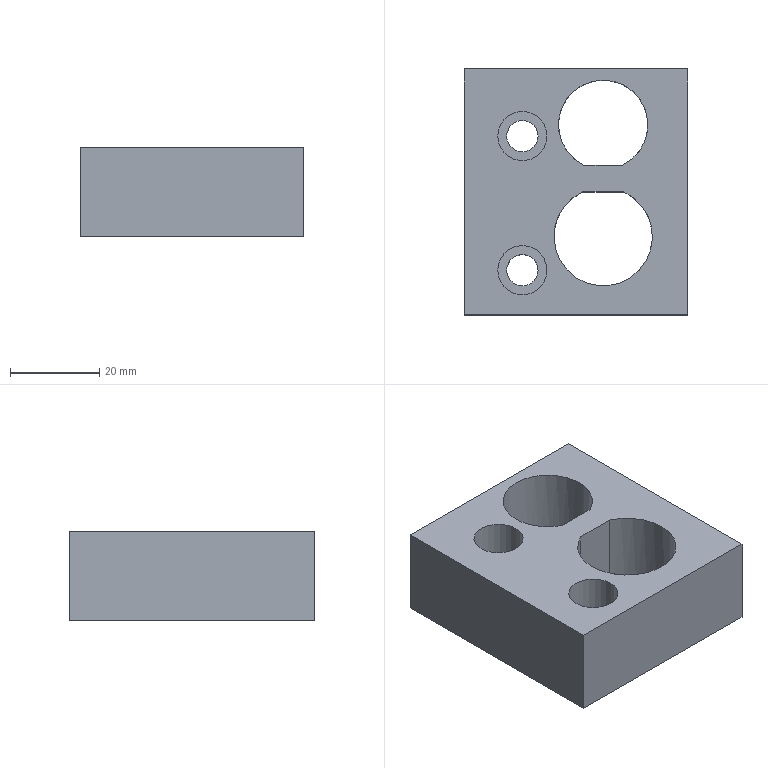Part | STEP file | lll_id690_x_t | 1 solid | 19 faces | box 50 x 55 x 20 mm | volume 38452 mm3 | plane 13 | cylinder 6 | commonest cylinder face diameters 7.009 x2 11.008 x2 20 x1 22 x1
STEP:
#1=CARTESIAN_POINT('',(395.083,-115.522,-20.));
#2=VERTEX_POINT('',#1);
#3=CARTESIAN_POINT('',(395.083,-108.297,-20.));
#4=VERTEX_POINT('',#3);
#5=CARTESIAN_POINT('',(395.083,-100.,-20.));
#6=DIRECTION('',(0.,1.,0.));
#7=VECTOR('',#6,1.);
#8=LINE('',#5,#7);
#9=EDGE_CURVE('',#2,#4,#8,.T.);
#10=ORIENTED_EDGE('',*,*,#9,.T.);
#11=CARTESIAN_POINT('',(383.917,-108.297,-20.));
#12=VERTEX_POINT('',#11);
#13=CARTESIAN_POINT('',(389.5,-100.,-20.));
#14=DIRECTION('',(0.,0.,1.));
#15=DIRECTION('',(-1.,0.,0.));
#16=AXIS2_PLACEMENT_3D('',#13,#14,#15);
#17=CIRCLE('',#16,10.);
#18=EDGE_CURVE('',#4,#12,#17,.T.);
#19=ORIENTED_EDGE('',*,*,#18,.T.);
#20=CARTESIAN_POINT('',(383.917,-115.522,-20.));
#21=VERTEX_POINT('',#20);
#22=CARTESIAN_POINT('',(383.917,-100.,-20.));
#23=DIRECTION('',(0.,1.,0.));
#24=VECTOR('',#23,1.);
#25=LINE('',#22,#24);
#26=EDGE_CURVE('',#21,#12,#25,.T.);
#27=ORIENTED_EDGE('',*,*,#26,.F.);
#28=CARTESIAN_POINT('',(389.5,-125.,-20.));
#29=DIRECTION('',(0.,0.,-1.));
#30=DIRECTION('',(1.,0.,0.));
#31=AXIS2_PLACEMENT_3D('',#28,#29,#30);
#32=CIRCLE('',#31,11.);
#33=EDGE_CURVE('',#2,#21,#32,.T.);
#34=ORIENTED_EDGE('',*,*,#33,.F.);
#35=EDGE_LOOP('',(#10,#19,#27,#34));
#36=FACE_BOUND('',#35,.T.);
#37=CARTESIAN_POINT('',(367.916,-102.5,-20.));
#38=VERTEX_POINT('',#37);
#39=CARTESIAN_POINT('',(371.42,-102.5,-20.));
#40=DIRECTION('',(0.,0.,1.));
#41=DIRECTION('',(-1.,0.,0.));
#42=AXIS2_PLACEMENT_3D('',#39,#40,#41);
#43=CIRCLE('',#42,3.505);
#44=EDGE_CURVE('',#38,#38,#43,.T.);
#45=ORIENTED_EDGE('',*,*,#44,.T.);
#46=EDGE_LOOP('',(#45));
#47=FACE_BOUND('',#46,.T.);
#48=CARTESIAN_POINT('',(367.916,-132.5,-20.));
#49=VERTEX_POINT('',#48);
#50=CARTESIAN_POINT('',(371.42,-132.5,-20.));
#51=DIRECTION('',(0.,0.,1.));
#52=DIRECTION('',(-1.,0.,0.));
#53=AXIS2_PLACEMENT_3D('',#50,#51,#52);
#54=CIRCLE('',#53,3.505);
#55=EDGE_CURVE('',#49,#49,#54,.T.);
#56=ORIENTED_EDGE('',*,*,#55,.T.);
#57=EDGE_LOOP('',(#56));
#58=FACE_BOUND('',#57,.T.);
#59=CARTESIAN_POINT('',(408.42,-87.5,-20.));
#60=VERTEX_POINT('',#59);
#61=CARTESIAN_POINT('',(408.42,-142.5,-20.));
#62=VERTEX_POINT('',#61);
#63=CARTESIAN_POINT('',(408.42,-111.868,-20.));
#64=DIRECTION('',(0.,-1.,0.));
#65=VECTOR('',#64,1.);
#66=LINE('',#63,#65);
#67=EDGE_CURVE('',#60,#62,#66,.T.);
#68=ORIENTED_EDGE('',*,*,#67,.T.);
#69=CARTESIAN_POINT('',(358.42,-142.5,-20.));
#70=VERTEX_POINT('',#69);
#71=CARTESIAN_POINT('',(389.5,-142.5,-20.));
#72=DIRECTION('',(-1.,0.,0.));
#73=VECTOR('',#72,1.);
#74=LINE('',#71,#73);
#75=EDGE_CURVE('',#62,#70,#74,.T.);
#76=ORIENTED_EDGE('',*,*,#75,.T.);
#77=CARTESIAN_POINT('',(358.42,-87.5,-20.));
#78=VERTEX_POINT('',#77);
#79=CARTESIAN_POINT('',(358.42,-100.,-20.));
#80=DIRECTION('',(0.,1.,0.));
#81=VECTOR('',#80,1.);
#82=LINE('',#79,#81);
#83=EDGE_CURVE('',#70,#78,#82,.T.);
#84=ORIENTED_EDGE('',*,*,#83,.T.);
#85=CARTESIAN_POINT('',(389.5,-87.5,-20.));
#86=DIRECTION('',(1.,0.,0.));
#87=VECTOR('',#86,1.);
#88=LINE('',#85,#87);
#89=EDGE_CURVE('',#78,#60,#88,.T.);
#90=ORIENTED_EDGE('',*,*,#89,.T.);
#91=EDGE_LOOP('',(#68,#76,#84,#90));
#92=FACE_BOUND('',#91,.T.);
#93=CARTESIAN_POINT('',(389.5,-100.,-20.));
#94=DIRECTION('',(0.,0.,-1.));
#95=DIRECTION('',(-1.,0.,0.));
#96=AXIS2_PLACEMENT_3D('',#93,#94,#95);
#97=PLANE('',#96);
#98=ADVANCED_FACE('',(#36,#47,#58,#92),#97,.T.);
#99=CARTESIAN_POINT('',(376.924,-102.5,0.));
#100=VERTEX_POINT('',#99);
#101=CARTESIAN_POINT('',(371.42,-102.5,0.));
#102=DIRECTION('',(0.,0.,-1.));
#103=DIRECTION('',(1.,0.,0.));
#104=AXIS2_PLACEMENT_3D('',#101,#102,#103);
#105=CIRCLE('',#104,5.504);
#106=EDGE_CURVE('',#100,#100,#105,.T.);
#107=ORIENTED_EDGE('',*,*,#106,.T.);
#108=EDGE_LOOP('',(#107));
#109=FACE_BOUND('',#108,.T.);
#110=CARTESIAN_POINT('',(376.924,-132.5,0.));
#111=VERTEX_POINT('',#110);
#112=CARTESIAN_POINT('',(371.42,-132.5,0.));
#113=DIRECTION('',(0.,0.,-1.));
#114=DIRECTION('',(1.,0.,0.));
#115=AXIS2_PLACEMENT_3D('',#112,#113,#114);
#116=CIRCLE('',#115,5.504);
#117=EDGE_CURVE('',#111,#111,#116,.T.);
#118=ORIENTED_EDGE('',*,*,#117,.T.);
#119=EDGE_LOOP('',(#118));
#120=FACE_BOUND('',#119,.T.);
#121=CARTESIAN_POINT('',(408.42,-87.5,0.));
#122=VERTEX_POINT('',#121);
#123=CARTESIAN_POINT('',(358.42,-87.5,0.));
#124=VERTEX_POINT('',#123);
#125=CARTESIAN_POINT('',(389.5,-87.5,0.));
#126=DIRECTION('',(-1.,0.,0.));
#127=VECTOR('',#126,1.);
#128=LINE('',#125,#127);
#129=EDGE_CURVE('',#122,#124,#128,.T.);
#130=ORIENTED_EDGE('',*,*,#129,.T.);
#131=CARTESIAN_POINT('',(358.42,-142.5,0.));
#132=VERTEX_POINT('',#131);
#133=CARTESIAN_POINT('',(358.42,-100.,0.));
#134=DIRECTION('',(0.,-1.,0.));
#135=VECTOR('',#134,1.);
#136=LINE('',#133,#135);
#137=EDGE_CURVE('',#124,#132,#136,.T.);
#138=ORIENTED_EDGE('',*,*,#137,.T.);
#139=CARTESIAN_POINT('',(408.42,-142.5,0.));
#140=VERTEX_POINT('',#139);
#141=CARTESIAN_POINT('',(389.5,-142.5,0.));
#142=DIRECTION('',(1.,0.,0.));
#143=VECTOR('',#142,1.);
#144=LINE('',#141,#143);
#145=EDGE_CURVE('',#132,#140,#144,.T.);
#146=ORIENTED_EDGE('',*,*,#145,.T.);
#147=CARTESIAN_POINT('',(408.42,-111.868,0.));
#148=DIRECTION('',(0.,1.,0.));
#149=VECTOR('',#148,1.);
#150=LINE('',#147,#149);
#151=EDGE_CURVE('',#140,#122,#150,.T.);
#152=ORIENTED_EDGE('',*,*,#151,.T.);
#153=EDGE_LOOP('',(#130,#138,#146,#152));
#154=FACE_BOUND('',#153,.T.);
#155=CARTESIAN_POINT('',(385.141,-109.,0.));
#156=VERTEX_POINT('',#155);
#157=CARTESIAN_POINT('',(393.859,-109.,0.));
#158=VERTEX_POINT('',#157);
#159=CARTESIAN_POINT('',(389.5,-100.,0.));
#160=DIRECTION('',(0.,0.,-1.));
#161=DIRECTION('',(1.,0.,0.));
#162=AXIS2_PLACEMENT_3D('',#159,#160,#161);
#163=CIRCLE('',#162,10.);
#164=EDGE_CURVE('',#156,#158,#163,.T.);
#165=ORIENTED_EDGE('',*,*,#164,.T.);
#166=CARTESIAN_POINT('',(389.5,-109.,0.));
#167=DIRECTION('',(1.,0.,0.));
#168=VECTOR('',#167,1.);
#169=LINE('',#166,#168);
#170=EDGE_CURVE('',#156,#158,#169,.T.);
#171=ORIENTED_EDGE('',*,*,#170,.F.);
#172=EDGE_LOOP('',(#165,#171));
#173=FACE_BOUND('',#172,.T.);
#174=CARTESIAN_POINT('',(384.917,-115.,0.));
#175=VERTEX_POINT('',#174);
#176=CARTESIAN_POINT('',(394.083,-115.,0.));
#177=VERTEX_POINT('',#176);
#178=CARTESIAN_POINT('',(389.5,-115.,0.));
#179=DIRECTION('',(1.,0.,0.));
#180=VECTOR('',#179,1.);
#181=LINE('',#178,#180);
#182=EDGE_CURVE('',#175,#177,#181,.T.);
#183=ORIENTED_EDGE('',*,*,#182,.T.);
#184=CARTESIAN_POINT('',(389.5,-125.,0.));
#185=DIRECTION('',(0.,0.,1.));
#186=DIRECTION('',(1.,0.,0.));
#187=AXIS2_PLACEMENT_3D('',#184,#185,#186);
#188=CIRCLE('',#187,11.);
#189=EDGE_CURVE('',#175,#177,#188,.T.);
#190=ORIENTED_EDGE('',*,*,#189,.F.);
#191=EDGE_LOOP('',(#183,#190));
#192=FACE_BOUND('',#191,.T.);
#193=CARTESIAN_POINT('',(389.5,-100.,0.));
#194=DIRECTION('',(0.,0.,1.));
#195=DIRECTION('',(1.,0.,0.));
#196=AXIS2_PLACEMENT_3D('',#193,#194,#195);
#197=PLANE('',#196);
#198=ADVANCED_FACE('',(#109,#120,#154,#173,#192),#197,.T.);
#199=CARTESIAN_POINT('',(358.42,-87.5,-20.));
#200=DIRECTION('',(0.,0.,1.));
#201=VECTOR('',#200,1.);
#202=LINE('',#199,#201);
#203=EDGE_CURVE('',#78,#124,#202,.T.);
#204=ORIENTED_EDGE('',*,*,#203,.F.);
#205=ORIENTED_EDGE('',*,*,#83,.F.);
#206=CARTESIAN_POINT('',(358.42,-142.5,-20.));
#207=DIRECTION('',(0.,0.,1.));
#208=VECTOR('',#207,1.);
#209=LINE('',#206,#208);
#210=EDGE_CURVE('',#70,#132,#209,.T.);
#211=ORIENTED_EDGE('',*,*,#210,.T.);
#212=ORIENTED_EDGE('',*,*,#137,.F.);
#213=EDGE_LOOP('',(#204,#205,#211,#212));
#214=FACE_OUTER_BOUND('',#213,.T.);
#215=CARTESIAN_POINT('',(358.42,-100.,-20.));
#216=DIRECTION('',(-1.,0.,0.));
#217=DIRECTION('',(0.,0.,1.));
#218=AXIS2_PLACEMENT_3D('',#215,#216,#217);
#219=PLANE('',#218);
#220=ADVANCED_FACE('',(#214),#219,.T.);
#221=CARTESIAN_POINT('',(408.42,-87.5,-20.));
#222=DIRECTION('',(0.,0.,1.));
#223=VECTOR('',#222,1.);
#224=LINE('',#221,#223);
#225=EDGE_CURVE('',#60,#122,#224,.T.);
#226=ORIENTED_EDGE('',*,*,#225,.F.);
#227=ORIENTED_EDGE('',*,*,#89,.F.);
#228=ORIENTED_EDGE('',*,*,#203,.T.);
#229=ORIENTED_EDGE('',*,*,#129,.F.);
#230=EDGE_LOOP('',(#226,#227,#228,#229));
#231=FACE_OUTER_BOUND('',#230,.T.);
#232=CARTESIAN_POINT('',(389.5,-87.5,-20.));
#233=DIRECTION('',(0.,1.,0.));
#234=DIRECTION('',(0.,0.,-1.));
#235=AXIS2_PLACEMENT_3D('',#232,#233,#234);
#236=PLANE('',#235);
#237=ADVANCED_FACE('',(#231),#236,.T.);
#238=ORIENTED_EDGE('',*,*,#67,.F.);
#239=ORIENTED_EDGE('',*,*,#225,.T.);
#240=ORIENTED_EDGE('',*,*,#151,.F.);
#241=CARTESIAN_POINT('',(408.42,-142.5,-16.5));
#242=DIRECTION('',(0.,0.,1.));
#243=VECTOR('',#242,1.);
#244=LINE('',#241,#243);
#245=EDGE_CURVE('',#62,#140,#244,.T.);
#246=ORIENTED_EDGE('',*,*,#245,.F.);
#247=EDGE_LOOP('',(#238,#239,#240,#246));
#248=FACE_OUTER_BOUND('',#247,.T.);
#249=CARTESIAN_POINT('',(408.42,-111.868,-16.5));
#250=DIRECTION('',(1.,0.,0.));
#251=DIRECTION('',(0.,0.,-1.));
#252=AXIS2_PLACEMENT_3D('',#249,#250,#251);
#253=PLANE('',#252);
#254=ADVANCED_FACE('',(#248),#253,.T.);
#255=CARTESIAN_POINT('',(395.083,-108.297,-15.));
#256=VERTEX_POINT('',#255);
#257=CARTESIAN_POINT('',(393.859,-109.,-15.));
#258=VERTEX_POINT('',#257);
#259=CARTESIAN_POINT('',(389.5,-100.,-15.));
#260=DIRECTION('',(0.,0.,-1.));
#261=DIRECTION('',(1.,0.,0.));
#262=AXIS2_PLACEMENT_3D('',#259,#260,#261);
#263=CIRCLE('',#262,10.);
#264=EDGE_CURVE('',#256,#258,#263,.T.);
#265=ORIENTED_EDGE('',*,*,#264,.T.);
#266=CARTESIAN_POINT('',(393.859,-109.,-15.));
#267=DIRECTION('',(0.,0.,1.));
#268=VECTOR('',#267,1.);
#269=LINE('',#266,#268);
#270=EDGE_CURVE('',#258,#158,#269,.T.);
#271=ORIENTED_EDGE('',*,*,#270,.T.);
#272=ORIENTED_EDGE('',*,*,#164,.F.);
#273=CARTESIAN_POINT('',(385.141,-109.,-15.));
#274=VERTEX_POINT('',#273);
#275=CARTESIAN_POINT('',(385.141,-109.,0.));
#276=DIRECTION('',(0.,0.,-1.));
#277=VECTOR('',#276,1.);
#278=LINE('',#275,#277);
#279=EDGE_CURVE('',#156,#274,#278,.T.);
#280=ORIENTED_EDGE('',*,*,#279,.T.);
#281=CARTESIAN_POINT('',(383.917,-108.297,-15.));
#282=VERTEX_POINT('',#281);
#283=CARTESIAN_POINT('',(389.5,-100.,-15.));
#284=DIRECTION('',(0.,0.,-1.));
#285=DIRECTION('',(1.,0.,0.));
#286=AXIS2_PLACEMENT_3D('',#283,#284,#285);
#287=CIRCLE('',#286,10.);
#288=EDGE_CURVE('',#274,#282,#287,.T.);
#289=ORIENTED_EDGE('',*,*,#288,.T.);
#290=CARTESIAN_POINT('',(383.917,-108.297,0.));
#291=DIRECTION('',(0.,0.,-1.));
#292=VECTOR('',#291,1.);
#293=LINE('',#290,#292);
#294=EDGE_CURVE('',#282,#12,#293,.T.);
#295=ORIENTED_EDGE('',*,*,#294,.T.);
#296=ORIENTED_EDGE('',*,*,#18,.F.);
#297=CARTESIAN_POINT('',(395.083,-108.297,0.));
#298=DIRECTION('',(0.,0.,-1.));
#299=VECTOR('',#298,1.);
#300=LINE('',#297,#299);
#301=EDGE_CURVE('',#256,#4,#300,.T.);
#302=ORIENTED_EDGE('',*,*,#301,.F.);
#303=EDGE_LOOP('',(#265,#271,#272,#280,#289,#295,#296,#302));
#304=FACE_OUTER_BOUND('',#303,.T.);
#305=CARTESIAN_POINT('',(389.5,-100.,0.));
#306=DIRECTION('',(0.,0.,-1.));
#307=DIRECTION('',(1.,0.,0.));
#308=AXIS2_PLACEMENT_3D('',#305,#306,#307);
#309=CYLINDRICAL_SURFACE('',#308,10.);
#310=ADVANCED_FACE('',(#304),#309,.F.);
#311=CARTESIAN_POINT('',(389.5,-109.,-15.));
#312=DIRECTION('',(-1.,0.,0.));
#313=VECTOR('',#312,1.);
#314=LINE('',#311,#313);
#315=EDGE_CURVE('',#258,#274,#314,.T.);
#316=ORIENTED_EDGE('',*,*,#315,.T.);
#317=ORIENTED_EDGE('',*,*,#279,.F.);
#318=ORIENTED_EDGE('',*,*,#170,.T.);
#319=ORIENTED_EDGE('',*,*,#270,.F.);
#320=EDGE_LOOP('',(#316,#317,#318,#319));
#321=FACE_OUTER_BOUND('',#320,.T.);
#322=CARTESIAN_POINT('',(389.5,-109.,-10.));
#323=DIRECTION('',(0.,1.,0.));
#324=DIRECTION('',(0.,0.,1.));
#325=AXIS2_PLACEMENT_3D('',#322,#323,#324);
#326=PLANE('',#325);
#327=ADVANCED_FACE('',(#321),#326,.T.);
#328=ORIENTED_EDGE('',*,*,#210,.F.);
#329=ORIENTED_EDGE('',*,*,#75,.F.);
#330=ORIENTED_EDGE('',*,*,#245,.T.);
#331=ORIENTED_EDGE('',*,*,#145,.F.);
#332=EDGE_LOOP('',(#328,#329,#330,#331));
#333=FACE_OUTER_BOUND('',#332,.T.);
#334=CARTESIAN_POINT('',(389.5,-142.5,-20.));
#335=DIRECTION('',(0.,-1.,0.));
#336=DIRECTION('',(0.,0.,1.));
#337=AXIS2_PLACEMENT_3D('',#334,#335,#336);
#338=PLANE('',#337);
#339=ADVANCED_FACE('',(#333),#338,.T.);
#340=ORIENTED_EDGE('',*,*,#33,.T.);
#341=CARTESIAN_POINT('',(383.917,-115.522,-15.));
#342=VERTEX_POINT('',#341);
#343=CARTESIAN_POINT('',(383.917,-115.522,0.));
#344=DIRECTION('',(0.,0.,1.));
#345=VECTOR('',#344,1.);
#346=LINE('',#343,#345);
#347=EDGE_CURVE('',#21,#342,#346,.T.);
#348=ORIENTED_EDGE('',*,*,#347,.T.);
#349=CARTESIAN_POINT('',(384.917,-115.,-15.));
#350=VERTEX_POINT('',#349);
#351=CARTESIAN_POINT('',(389.5,-125.,-15.));
#352=DIRECTION('',(0.,0.,-1.));
#353=DIRECTION('',(1.,0.,0.));
#354=AXIS2_PLACEMENT_3D('',#351,#352,#353);
#355=CIRCLE('',#354,11.);
#356=EDGE_CURVE('',#342,#350,#355,.T.);
#357=ORIENTED_EDGE('',*,*,#356,.T.);
#358=CARTESIAN_POINT('',(384.917,-115.,0.));
#359=DIRECTION('',(0.,0.,-1.));
#360=VECTOR('',#359,1.);
#361=LINE('',#358,#360);
#362=EDGE_CURVE('',#175,#350,#361,.T.);
#363=ORIENTED_EDGE('',*,*,#362,.F.);
#364=ORIENTED_EDGE('',*,*,#189,.T.);
#365=CARTESIAN_POINT('',(394.083,-115.,-15.));
#366=VERTEX_POINT('',#365);
#367=CARTESIAN_POINT('',(394.083,-115.,0.));
#368=DIRECTION('',(0.,0.,1.));
#369=VECTOR('',#368,1.);
#370=LINE('',#367,#369);
#371=EDGE_CURVE('',#366,#177,#370,.T.);
#372=ORIENTED_EDGE('',*,*,#371,.F.);
#373=CARTESIAN_POINT('',(395.083,-115.522,-15.));
#374=VERTEX_POINT('',#373);
#375=CARTESIAN_POINT('',(389.5,-125.,-15.));
#376=DIRECTION('',(0.,0.,-1.));
#377=DIRECTION('',(1.,0.,0.));
#378=AXIS2_PLACEMENT_3D('',#375,#376,#377);
#379=CIRCLE('',#378,11.);
#380=EDGE_CURVE('',#366,#374,#379,.T.);
#381=ORIENTED_EDGE('',*,*,#380,.T.);
#382=CARTESIAN_POINT('',(395.083,-115.522,0.));
#383=DIRECTION('',(0.,0.,1.));
#384=VECTOR('',#383,1.);
#385=LINE('',#382,#384);
#386=EDGE_CURVE('',#2,#374,#385,.T.);
#387=ORIENTED_EDGE('',*,*,#386,.F.);
#388=EDGE_LOOP('',(#340,#348,#357,#363,#364,#372,#381,#387));
#389=FACE_OUTER_BOUND('',#388,.T.);
#390=CARTESIAN_POINT('',(389.5,-125.,0.));
#391=DIRECTION('',(0.,0.,-1.));
#392=DIRECTION('',(-1.,0.,0.));
#393=AXIS2_PLACEMENT_3D('',#390,#391,#392);
#394=CYLINDRICAL_SURFACE('',#393,11.);
#395=ADVANCED_FACE('',(#389),#394,.F.);
#396=CARTESIAN_POINT('',(389.5,-115.,-15.));
#397=DIRECTION('',(1.,0.,0.));
#398=VECTOR('',#397,1.);
#399=LINE('',#396,#398);
#400=EDGE_CURVE('',#350,#366,#399,.T.);
#401=ORIENTED_EDGE('',*,*,#400,.T.);
#402=ORIENTED_EDGE('',*,*,#371,.T.);
#403=ORIENTED_EDGE('',*,*,#182,.F.);
#404=ORIENTED_EDGE('',*,*,#362,.T.);
#405=EDGE_LOOP('',(#401,#402,#403,#404));
#406=FACE_OUTER_BOUND('',#405,.T.);
#407=CARTESIAN_POINT('',(389.5,-115.,-10.));
#408=DIRECTION('',(0.,-1.,0.));
#409=DIRECTION('',(0.,0.,1.));
#410=AXIS2_PLACEMENT_3D('',#407,#408,#409);
#411=PLANE('',#410);
#412=ADVANCED_FACE('',(#406),#411,.T.);
#413=ORIENTED_EDGE('',*,*,#400,.F.);
#414=ORIENTED_EDGE('',*,*,#356,.F.);
#415=CARTESIAN_POINT('',(383.917,-115.,-15.));
#416=DIRECTION('',(0.,1.,0.));
#417=VECTOR('',#416,1.);
#418=LINE('',#415,#417);
#419=EDGE_CURVE('',#342,#282,#418,.T.);
#420=ORIENTED_EDGE('',*,*,#419,.T.);
#421=ORIENTED_EDGE('',*,*,#288,.F.);
#422=ORIENTED_EDGE('',*,*,#315,.F.);
#423=ORIENTED_EDGE('',*,*,#264,.F.);
#424=CARTESIAN_POINT('',(395.083,-115.,-15.));
#425=DIRECTION('',(0.,1.,0.));
#426=VECTOR('',#425,1.);
#427=LINE('',#424,#426);
#428=EDGE_CURVE('',#374,#256,#427,.T.);
#429=ORIENTED_EDGE('',*,*,#428,.F.);
#430=ORIENTED_EDGE('',*,*,#380,.F.);
#431=EDGE_LOOP('',(#413,#414,#420,#421,#422,#423,#429,#430));
#432=FACE_OUTER_BOUND('',#431,.T.);
#433=CARTESIAN_POINT('',(389.5,-125.,-15.));
#434=DIRECTION('',(0.,0.,1.));
#435=DIRECTION('',(1.,0.,0.));
#436=AXIS2_PLACEMENT_3D('',#433,#434,#435);
#437=PLANE('',#436);
#438=ADVANCED_FACE('',(#432),#437,.F.);
#439=ORIENTED_EDGE('',*,*,#55,.F.);
#440=EDGE_LOOP('',(#439));
#441=FACE_BOUND('',#440,.T.);
#442=CARTESIAN_POINT('',(367.916,-132.5,-9.));
#443=VERTEX_POINT('',#442);
#444=CARTESIAN_POINT('',(371.42,-132.5,-9.));
#445=DIRECTION('',(0.,0.,1.));
#446=DIRECTION('',(-1.,0.,0.));
#447=AXIS2_PLACEMENT_3D('',#444,#445,#446);
#448=CIRCLE('',#447,3.505);
#449=EDGE_CURVE('',#443,#443,#448,.T.);
#450=ORIENTED_EDGE('',*,*,#449,.T.);
#451=EDGE_LOOP('',(#450));
#452=FACE_BOUND('',#451,.T.);
#453=CARTESIAN_POINT('',(371.42,-132.5,2.));
#454=DIRECTION('',(0.,0.,-1.));
#455=DIRECTION('',(1.,0.,0.));
#456=AXIS2_PLACEMENT_3D('',#453,#454,#455);
#457=CYLINDRICAL_SURFACE('',#456,3.505);
#458=ADVANCED_FACE('',(#441,#452),#457,.F.);
#459=ORIENTED_EDGE('',*,*,#449,.F.);
#460=EDGE_LOOP('',(#459));
#461=FACE_BOUND('',#460,.T.);
#462=CARTESIAN_POINT('',(365.916,-132.5,-9.));
#463=VERTEX_POINT('',#462);
#464=CARTESIAN_POINT('',(371.42,-132.5,-9.));
#465=DIRECTION('',(0.,0.,1.));
#466=DIRECTION('',(-1.,0.,0.));
#467=AXIS2_PLACEMENT_3D('',#464,#465,#466);
#468=CIRCLE('',#467,5.504);
#469=EDGE_CURVE('',#463,#463,#468,.T.);
#470=ORIENTED_EDGE('',*,*,#469,.T.);
#471=EDGE_LOOP('',(#470));
#472=FACE_BOUND('',#471,.T.);
#473=CARTESIAN_POINT('',(371.42,-132.5,-9.));
#474=DIRECTION('',(0.,0.,-1.));
#475=DIRECTION('',(1.,0.,0.));
#476=AXIS2_PLACEMENT_3D('',#473,#474,#475);
#477=PLANE('',#476);
#478=ADVANCED_FACE('',(#461,#472),#477,.F.);
#479=ORIENTED_EDGE('',*,*,#117,.F.);
#480=EDGE_LOOP('',(#479));
#481=FACE_BOUND('',#480,.T.);
#482=ORIENTED_EDGE('',*,*,#469,.F.);
#483=EDGE_LOOP('',(#482));
#484=FACE_BOUND('',#483,.T.);
#485=CARTESIAN_POINT('',(371.42,-132.5,0.000025));
#486=DIRECTION('',(0.,0.,-1.));
#487=DIRECTION('',(1.,0.,0.));
#488=AXIS2_PLACEMENT_3D('',#485,#486,#487);
#489=CYLINDRICAL_SURFACE('',#488,5.504);
#490=ADVANCED_FACE('',(#481,#484),#489,.F.);
#491=ORIENTED_EDGE('',*,*,#44,.F.);
#492=EDGE_LOOP('',(#491));
#493=FACE_BOUND('',#492,.T.);
#494=CARTESIAN_POINT('',(367.916,-102.5,-9.));
#495=VERTEX_POINT('',#494);
#496=CARTESIAN_POINT('',(371.42,-102.5,-9.));
#497=DIRECTION('',(0.,0.,1.));
#498=DIRECTION('',(-1.,0.,0.));
#499=AXIS2_PLACEMENT_3D('',#496,#497,#498);
#500=CIRCLE('',#499,3.505);
#501=EDGE_CURVE('',#495,#495,#500,.T.);
#502=ORIENTED_EDGE('',*,*,#501,.T.);
#503=EDGE_LOOP('',(#502));
#504=FACE_BOUND('',#503,.T.);
#505=CARTESIAN_POINT('',(371.42,-102.5,2.));
#506=DIRECTION('',(0.,0.,-1.));
#507=DIRECTION('',(1.,0.,0.));
#508=AXIS2_PLACEMENT_3D('',#505,#506,#507);
#509=CYLINDRICAL_SURFACE('',#508,3.505);
#510=ADVANCED_FACE('',(#493,#504),#509,.F.);
#511=ORIENTED_EDGE('',*,*,#501,.F.);
#512=EDGE_LOOP('',(#511));
#513=FACE_BOUND('',#512,.T.);
#514=CARTESIAN_POINT('',(365.916,-102.5,-9.));
#515=VERTEX_POINT('',#514);
#516=CARTESIAN_POINT('',(371.42,-102.5,-9.));
#517=DIRECTION('',(0.,0.,1.));
#518=DIRECTION('',(-1.,0.,0.));
#519=AXIS2_PLACEMENT_3D('',#516,#517,#518);
#520=CIRCLE('',#519,5.504);
#521=EDGE_CURVE('',#515,#515,#520,.T.);
#522=ORIENTED_EDGE('',*,*,#521,.T.);
#523=EDGE_LOOP('',(#522));
#524=FACE_BOUND('',#523,.T.);
#525=CARTESIAN_POINT('',(371.42,-102.5,-9.));
#526=DIRECTION('',(0.,0.,-1.));
#527=DIRECTION('',(1.,0.,0.));
#528=AXIS2_PLACEMENT_3D('',#525,#526,#527);
#529=PLANE('',#528);
#530=ADVANCED_FACE('',(#513,#524),#529,.F.);
#531=ORIENTED_EDGE('',*,*,#106,.F.);
#532=EDGE_LOOP('',(#531));
#533=FACE_BOUND('',#532,.T.);
#534=ORIENTED_EDGE('',*,*,#521,.F.);
#535=EDGE_LOOP('',(#534));
#536=FACE_BOUND('',#535,.T.);
#537=CARTESIAN_POINT('',(371.42,-102.5,0.000025));
#538=DIRECTION('',(0.,0.,-1.));
#539=DIRECTION('',(1.,0.,0.));
#540=AXIS2_PLACEMENT_3D('',#537,#538,#539);
#541=CYLINDRICAL_SURFACE('',#540,5.504);
#542=ADVANCED_FACE('',(#533,#536),#541,.F.);
#543=ORIENTED_EDGE('',*,*,#9,.F.);
#544=ORIENTED_EDGE('',*,*,#386,.T.);
#545=ORIENTED_EDGE('',*,*,#428,.T.);
#546=ORIENTED_EDGE('',*,*,#301,.T.);
#547=EDGE_LOOP('',(#543,#544,#545,#546));
#548=FACE_OUTER_BOUND('',#547,.T.);
#549=CARTESIAN_POINT('',(395.083,-115.,-33.));
#550=DIRECTION('',(1.,0.,0.));
#551=DIRECTION('',(0.,0.,1.));
#552=AXIS2_PLACEMENT_3D('',#549,#550,#551);
#553=PLANE('',#552);
#554=ADVANCED_FACE('',(#548),#553,.F.);
#555=ORIENTED_EDGE('',*,*,#347,.F.);
#556=ORIENTED_EDGE('',*,*,#26,.T.);
#557=ORIENTED_EDGE('',*,*,#294,.F.);
#558=ORIENTED_EDGE('',*,*,#419,.F.);
#559=EDGE_LOOP('',(#555,#556,#557,#558));
#560=FACE_OUTER_BOUND('',#559,.T.);
#561=CARTESIAN_POINT('',(383.917,-115.,-33.));
#562=DIRECTION('',(1.,0.,0.));
#563=DIRECTION('',(0.,0.,1.));
#564=AXIS2_PLACEMENT_3D('',#561,#562,#563);
#565=PLANE('',#564);
#566=ADVANCED_FACE('',(#560),#565,.T.);
#567=CLOSED_SHELL('',(#98,#198,#220,#237,#254,#310,#327,#339,#395,#412,#438,#458,#478,#490,#510,#530,#542,#554,#566));
#568=MANIFOLD_SOLID_BREP('',#567);
#569=(LENGTH_UNIT()NAMED_UNIT(*)SI_UNIT(.MILLI.,.METRE.));
#570=UNCERTAINTY_MEASURE_WITH_UNIT(LENGTH_MEASURE(0.00002),#569,'','');
#571=(NAMED_UNIT(*)PLANE_ANGLE_UNIT()SI_UNIT($,.RADIAN.));
#572=PLANE_ANGLE_MEASURE_WITH_UNIT(PLANE_ANGLE_MEASURE(0.01745),#571);
#573=DIMENSIONAL_EXPONENTS(0.,0.,0.,0.,0.,0.,0.);
#574=(CONVERSION_BASED_UNIT('DEGREE',#572)NAMED_UNIT(#573)PLANE_ANGLE_UNIT());
#575=(NAMED_UNIT(*)SI_UNIT($,.STERADIAN.)SOLID_ANGLE_UNIT());
#576=(GEOMETRIC_REPRESENTATION_CONTEXT(3)GLOBAL_UNCERTAINTY_ASSIGNED_CONTEXT((#570))GLOBAL_UNIT_ASSIGNED_CONTEXT((#569,#574,#575))REPRESENTATION_CONTEXT('',''));
#577=ADVANCED_BREP_SHAPE_REPRESENTATION('',(#568),#576);